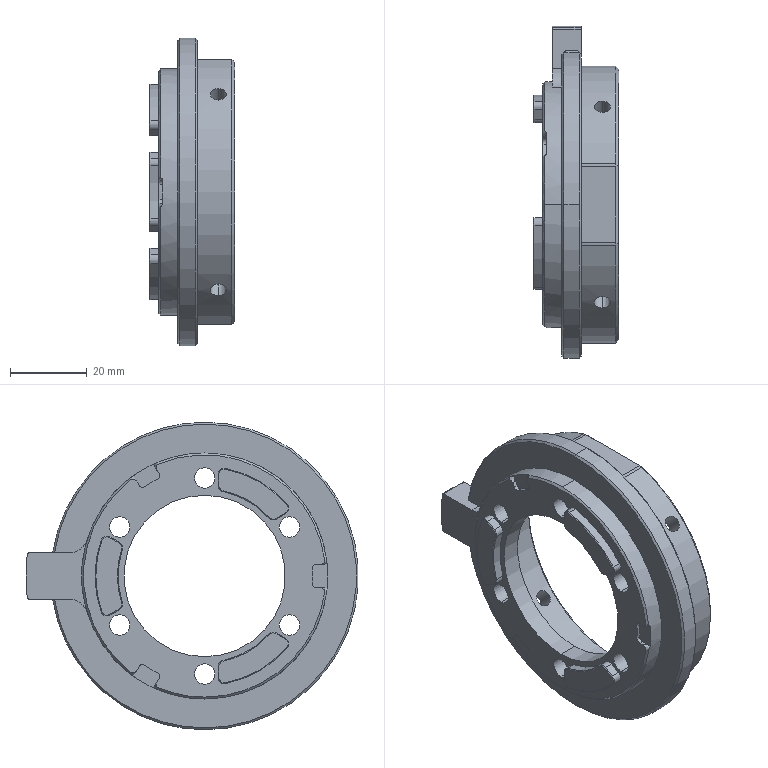NC program | NX | posted with a generic post | part box 22.3 x 86.5 x 80 mm
Lines 3855 to 5076 of 5076:
(ZLEVEL_PROFILE_COPY_1_COPY_COPY_1 , TOOL : D10JING)
N7696 T14 M6
N7698 G54
N7700 G17 G0 G90 X-1.456 Y13.884 S9500 M3
N7702 G43 Z30. H14
N7704 Z-21.3
N7706 G94 G1 Z-22.3 F1000.
N7708 X-2.389 Y15.5
N7710 G3 X-3.255 Y16. R1.
N7712 X-19.255 Y0. R16. F1200.
N7714 X-3.255 Y16. R-16.
N7716 X-4.121 Y15.5 R1.
N7718 G1 X-5.054 Y13.884
N7720 Z-21.3
N7722 G0 Z53.
N7724 X44.033 Y-12.821
N7726 Z-21.3
N7728 G1 Z-22.3 F1000.
N7730 X43.27 Y-11.5
N7732 G3 X42.404 Y-11. R1.
N7734 G1 X40.38 F1200.
N7736 G2 X40.38 Y11. R-45.
N7738 G1 X42.404
N7740 G2 X47.862 Y6.18 R5.5
N7742 X47.862 Y-6.18 R50.
N7744 X42.404 Y-11. R5.5
N7746 G3 X41.538 Y-11.5 R1.
N7748 G1 X41.912 Y-13.
N7750 Z-21.3
N7752 G0 Z30.
(ZLEVEL_PROFILE_COPY_1_COPY_COPY_1_COPY , TOOL : D10JING)
N7754 X-1.485 Y23.935
N7756 Z-11.7
N7758 G1 Z-12.7 F1000.
N7760 X-2.389 Y25.5
N7762 G3 X-3.255 Y26. R1.
N7764 X-29.255 Y0. R26. F1200.
N7766 X-3.255 Y26. R-26.
N7768 X-4.121 Y25.5 R1.
N7770 G1 X-5.025 Y23.935
N7772 Z-11.7
N7774 G0 Z30.
(FLOOR_WALL_1 , TOOL : D10JING)
N7776 X-21.493 Y2.989
N7778 Z-11.8
N7780 G1 Z-14.8 F1250.
N7782 X-21.755 Y0.
N7784 G3 X-20.35 Y-7.071 R18.5
N7786 G2 X-19.676 Y-9.481 R10.5
N7788 X-17.926 Y-11.269 R10.5
N7790 G3 X-5.679 Y-18.341 R18.5
N7792 G2 X-3.255 Y-18.962 R10.5
N7794 X-0.831 Y-18.341 R10.5
N7796 G3 X11.417 Y-11.269 R18.5
N7798 G2 X13.166 Y-9.481 R10.5
N7800 X13.84 Y-7.071 R10.5
N7802 G3 X13.84 Y7.071 R18.5
N7804 G2 X13.166 Y9.481 R10.5
N7806 X11.417 Y11.269 R10.5
N7808 G3 X-0.831 Y18.341 R18.5
N7810 G2 X-3.255 Y18.962 R10.5
N7812 X-5.679 Y18.341 R10.5
N7814 G3 X-17.926 Y11.269 R18.5
N7816 G2 X-19.676 Y9.481 R10.5
N7818 X-20.35 Y7.071 R10.5
N7820 G3 X-21.755 Y0. R18.5
N7822 G1 X-26.755
N7824 G3 X-24.971 Y-8.982 R23.5
N7826 G2 X-24.709 Y-12.387 R5.5
N7828 X-21.891 Y-14.315 R5.5
N7830 G3 X-6.334 Y-23.297 R23.5
N7832 G2 X-3.255 Y-24.774 R5.5
N7834 X-0.176 Y-23.297 R5.5
N7836 G3 X15.382 Y-14.315 R23.5
N7838 G2 X18.2 Y-12.387 R5.5
N7840 X18.461 Y-8.982 R5.5
N7842 G3 X18.461 Y8.982 R23.5
N7844 G2 X18.2 Y12.387 R5.5
N7846 X15.382 Y14.315 R5.5
N7848 G3 X-0.176 Y23.297 R23.5
N7850 G2 X-3.255 Y24.774 R5.5
N7852 X-6.334 Y23.297 R5.5
N7854 G3 X-21.891 Y14.315 R23.5
N7856 G2 X-24.709 Y12.387 R5.5
N7858 X-24.971 Y8.982 R5.5
N7860 G3 X-26.755 Y0. R23.5
N7862 G1 X-23.755
N7864 X-27.255
N7866 G3 X-25.433 Y-9.173 R24.
N7868 G2 X-25.338 Y-12.75 R5.
N7870 X-22.288 Y-14.62 R5.
N7872 G3 X-6.399 Y-23.793 R24.
N7874 G2 X-3.255 Y-25.5 R5.
N7876 X-0.11 Y-23.793 R5.
N7878 G3 X15.778 Y-14.62 R24.
N7880 G2 X18.829 Y-12.75 R5.
N7882 X18.923 Y-9.173 R5.
N7884 G3 X18.923 Y9.173 R24.
N7886 G2 X18.829 Y12.75 R5.
N7888 X15.778 Y14.62 R5.
N7890 G3 X-0.11 Y23.793 R24.
N7892 G2 X-3.255 Y25.5 R5.
N7894 X-6.399 Y23.793 R5.
N7896 G3 X-22.288 Y14.62 R24.
N7898 G2 X-25.338 Y12.75 R5.
N7900 X-25.433 Y9.173 R5.
N7902 G3 X-27.255 Y0. R24.
N7904 G1 X-24.255
N7906 Z-11.8
N7908 G0 Z30.
(FLOOR_WALL_1_COPY , TOOL : D10JING)
N7910 X42.135 Y14.
N7912 Z-6.8
N7914 G1 Z-9.8
N7916 X41.134 Y6.
N7918 X39.864
N7920 G2 X37.846 Y6.425 R5.
N7922 X37.846 Y-6.425 R41.6
N7924 X39.864 Y-6. R5.
N7926 G1 X42.404
N7928 G3 X42.9 Y-5.562 R0.5
N7930 X42.9 Y5.562 R45.
N7932 X42.404 Y6. R0.5
N7934 G1 X41.134
N7936 Y11.
N7938 X39.864
N7940 G3 X39.864 Y-11. R-44.5
N7942 G1 X42.404
N7944 G3 X47.862 Y-6.18 R5.5
N7946 X47.862 Y6.18 R50.
N7948 X42.404 Y11. R5.5
N7950 G1 X41.134
N7952 X39.55 Y10.608
N7954 X36.639 Y9.886
N7956 G2 X8.996 Y-39.232 R41.1
N7958 X6.581 Y-39.6 R8.1
N7960 G1 X-13.091
N7962 G2 X-15.505 Y-39.232 R8.1
N7964 X-15.505 Y39.232 R41.1
N7966 X-13.091 Y39.6 R8.1
N7968 G1 X6.581
N7970 G2 X8.996 Y39.232 R8.1
N7972 X36.639 Y9.886 R41.1
N7974 G1 X40.036 Y10.728
N7976 Z-6.8
N7978 G0 Z30.
N7980 M5
(ZLEVEL_PROFILE_1 , TOOL : D4R0.5)
N7982 T17 M6
N7984 G54
N7986 G17 G0 G90 X-2.557 Y28.19 S9500 M3
N7988 G43 Z30. H17
N7990 Z-11.4
N7992 G94 G1 Z-12.9 F2500.
N7994 X-2.908 Y28.799
N7996 G3 X-3.255 Y28.999 R0.4
N7998 X-32.253 Y0. R28.999
N8000 X-3.255 Y28.999 R-28.999
N8002 G1 Z-13.
N8004 G2 X25.744 Y0. R28.998
N8006 X-3.255 Y28.999 R-28.998
N8008 G1 Z-13.1
N8010 G3 X-32.253 Y0. R28.998
N8012 X-3.255 Y28.999 R-28.998
N8014 G1 Z-13.2
N8016 G2 X25.744 Y0. R28.998
N8018 X-3.255 Y28.999 R-28.998
N8020 G1 Z-13.3
N8022 G3 X-32.253 Y0. R28.998
N8024 X-3.255 Y28.999 R-28.998
N8026 G1 Y28.997 Z-13.4
N8028 G2 X-2.41 Y28.984 R28.997
N8030 G1 X-2.128 Y28.975
N8032 G2 X-1.001 Y28.909 R28.997
N8034 G1 X-0.72 Y28.886
N8036 G2 X0.655 Y28.732 R28.997
N8038 G1 X0.689 Y28.727
N8040 G2 X1.816 Y28.55 R28.997
N8042 G1 X2.097 Y28.498
N8044 G2 X3.224 Y28.264 R28.997
N8046 G1 X3.787 Y28.129
N8048 G2 X4.691 Y27.887 R28.997
N8050 G1 X5.196 Y27.738
N8052 G2 X5.759 Y27.56 R28.997
N8054 G1 X6.604 Y27.269
N8056 G2 X9.421 Y26.079 R28.997
N8058 G1 X9.985 Y25.797
N8060 G2 X10.829 Y25.346 R28.997
N8062 G1 X11.393 Y25.025
N8064 G2 X12.245 Y24.507 R28.997
N8066 G1 X12.52 Y24.33
N8068 G2 X13.506 Y23.662 R28.997
N8070 G1 X13.647 Y23.562
N8072 G2 X20.307 Y16.901 R28.997
N8074 G1 X20.407 Y16.761
N8076 G2 X21.076 Y15.775 R28.997
N8078 G1 X21.252 Y15.499
N8080 G2 X21.77 Y14.648 R28.997
N8082 G1 X22.092 Y14.084
N8084 G2 X22.543 Y13.24 R28.997
N8086 G1 X22.661 Y13.007
N8088 G2 X24.014 Y9.859 R28.997
N8090 G1 X24.069 Y9.703
N8092 X24.305 Y9.014
N8094 G2 X24.483 Y8.451 R28.997
N8096 G1 X24.632 Y7.946
N8098 G2 X24.874 Y7.042 R28.997
N8100 G1 X25.009 Y6.479
N8102 G2 X25.244 Y5.352 R28.997
N8104 G1 X25.295 Y5.07
N8106 G2 X25.472 Y3.944 R28.997
N8108 G1 X25.477 Y3.91
N8110 G2 X25.631 Y2.535 R28.997
N8112 G1 X25.654 Y2.253
N8114 G2 X25.72 Y1.127 R28.997
N8116 G1 X25.73 Y0.845
N8118 G2 X25.73 Y-0.845 R28.997
N8120 G1 X25.72 Y-1.127
N8122 G2 X25.654 Y-2.253 R28.997
N8124 G1 X25.631 Y-2.535
N8126 G2 X25.477 Y-3.91 R28.997
N8128 G1 X25.472 Y-3.944
N8130 G2 X25.295 Y-5.07 R28.997
N8132 G1 X25.244 Y-5.352
N8134 G2 X25.009 Y-6.479 R28.997
N8136 G1 X24.874 Y-7.042
N8138 G2 X24.632 Y-7.946 R28.997
N8140 G1 X24.483 Y-8.451
N8142 G2 X24.305 Y-9.014 R28.997
N8144 G1 X24.014 Y-9.859
N8146 G2 X22.661 Y-13.007 R28.997
N8148 G1 X22.543 Y-13.24
N8150 G2 X22.092 Y-14.084 R28.997
N8152 G1 X21.77 Y-14.648
N8154 G2 X21.252 Y-15.499 R28.997
N8156 G1 X21.076 Y-15.775
N8158 G2 X20.407 Y-16.761 R28.997
N8160 G1 X20.307 Y-16.901
N8162 G2 X13.647 Y-23.562 R28.997
N8164 G1 X13.506 Y-23.662
N8166 G2 X12.52 Y-24.33 R28.997
N8168 G1 X12.245 Y-24.507
N8170 G2 X11.393 Y-25.025 R28.997
N8172 G1 X10.829 Y-25.346
N8174 G2 X9.985 Y-25.797 R28.997
N8176 G1 X9.753 Y-25.915
N8178 G2 X6.604 Y-27.269 R28.997
N8180 G1 X6.449 Y-27.323
N8182 X5.759 Y-27.56
N8184 G2 X5.196 Y-27.738 R28.997
N8186 G1 X4.691 Y-27.887
N8188 G2 X3.787 Y-28.129 R28.997
N8190 G1 X3.224 Y-28.264
N8192 G2 X2.097 Y-28.498 R28.997
N8194 G1 X1.816 Y-28.55
N8196 G2 X0.689 Y-28.727 R28.997
N8198 G1 X0.655 Y-28.732
N8200 G2 X-0.72 Y-28.886 R28.997
N8202 G1 X-1.001 Y-28.909
N8204 G2 X-2.128 Y-28.975 R28.997
N8206 G1 X-2.41 Y-28.984
N8208 G2 X-4.1 Y-28.984 R28.997
N8210 G1 X-4.382 Y-28.975
N8212 G2 X-5.508 Y-28.909 R28.997
N8214 G1 X-5.79 Y-28.886
N8216 G2 X-7.164 Y-28.732 R28.997
N8218 G1 X-7.198 Y-28.727
N8220 G2 X-8.325 Y-28.55 R28.997
N8222 G1 X-8.607 Y-28.498
N8224 G2 X-9.734 Y-28.264 R28.997
N8226 G1 X-10.297 Y-28.129
N8228 G2 X-11.2 Y-27.887 R28.997
N8230 G1 X-11.705 Y-27.738
N8232 G2 X-12.269 Y-27.56 R28.997
N8234 G1 X-13.114 Y-27.269
N8236 G2 X-16.262 Y-25.915 R28.997
N8238 G1 X-16.495 Y-25.797
N8240 G2 X-17.339 Y-25.346 R28.997
N8242 G1 X-17.903 Y-25.025
N8244 G2 X-18.754 Y-24.507 R28.997
N8246 G1 X-19.03 Y-24.33
N8248 G2 X-20.016 Y-23.662 R28.997
N8250 G1 X-20.156 Y-23.562
N8252 G2 X-26.816 Y-16.901 R28.997
N8254 G1 X-26.916 Y-16.761
N8256 G2 X-27.585 Y-15.775 R28.997
N8258 G1 X-27.761 Y-15.499
N8260 G2 X-28.28 Y-14.648 R28.997
N8262 G1 X-28.601 Y-14.084
N8264 G2 X-29.052 Y-13.24 R28.997
N8266 G1 X-29.334 Y-12.676
N8268 G2 X-30.524 Y-9.859 R28.997
N8270 G1 X-30.578 Y-9.703
N8272 X-30.815 Y-9.014
N8274 G2 X-30.993 Y-8.451 R28.997
N8276 G1 X-31.142 Y-7.946
N8278 G2 X-31.383 Y-7.042 R28.997
N8280 G1 X-31.518 Y-6.479
N8282 G2 X-31.753 Y-5.352 R28.997
N8284 G1 X-31.805 Y-5.07
N8286 G2 X-31.982 Y-3.944 R28.997
N8288 G1 X-31.987 Y-3.91
N8290 G2 X-32.14 Y-2.535 R28.997
N8292 G1 X-32.164 Y-2.253
N8294 G2 X-32.23 Y-1.127 R28.997
N8296 G1 X-32.239 Y-0.845
N8298 G2 X-32.239 Y0.845 R28.997
N8300 G1 X-32.23 Y1.127
N8302 G2 X-31.987 Y3.91 R28.997
N8304 G1 X-31.982 Y3.944
N8306 G2 X-31.805 Y5.07 R28.997
N8308 G1 X-31.753 Y5.352
N8310 G2 X-31.518 Y6.479 R28.997
N8312 G1 X-31.383 Y7.042
N8314 G2 X-31.142 Y7.946 R28.997
N8316 G1 X-30.993 Y8.451
N8318 G2 X-30.815 Y9.014 R28.997
N8320 G1 X-30.524 Y9.859
N8322 G2 X-29.334 Y12.676 R28.997
N8324 G1 X-29.052 Y13.24
N8326 G2 X-28.601 Y14.084 R28.997
N8328 G1 X-28.28 Y14.648
N8330 G2 X-27.761 Y15.499 R28.997
N8332 G1 X-27.585 Y15.775
N8334 G2 X-26.916 Y16.761 R28.997
N8336 G1 X-26.816 Y16.901
N8338 G2 X-20.156 Y23.562 R28.997
N8340 G1 X-20.016 Y23.662
N8342 G2 X-19.03 Y24.33 R28.997
N8344 G1 X-18.754 Y24.507
N8346 G2 X-17.903 Y25.025 R28.997
N8348 G1 X-17.339 Y25.346
N8350 G2 X-16.495 Y25.797 R28.997
N8352 G1 X-15.931 Y26.079
N8354 G2 X-13.114 Y27.269 R28.997
N8356 G1 X-12.958 Y27.323
N8358 X-12.269 Y27.56
N8360 G2 X-11.705 Y27.738 R28.997
N8362 G1 X-11.2 Y27.887
N8364 G2 X-10.297 Y28.129 R28.997
N8366 G1 X-9.734 Y28.264
N8368 G2 X-8.607 Y28.498 R28.997
N8370 G1 X-8.325 Y28.55
N8372 G2 X-7.198 Y28.727 R28.997
N8374 G1 X-7.164 Y28.732
N8376 G2 X-5.79 Y28.886 R28.997
N8378 G1 X-5.508 Y28.909
N8380 G2 X-4.382 Y28.975 R28.997
N8382 G1 X-4.1 Y28.984
N8384 G2 X-3.255 Y28.997 R28.997
N8386 G1 Y28.987 Z-13.499
N8388 G3 X-32.242 Y0. R28.987
N8390 X-3.255 Y28.987 R-28.987
N8392 G1 Y28.979 Z-13.549
N8394 Y28.97 Z-13.598
N8396 X-3.246
N8398 G2 X25.715 Y-0.009 R28.97
N8400 X-3.255 Y28.97 R-28.97
N8402 G1 Y28.959 Z-13.646
N8404 Y28.947 Z-13.695
N8406 X-3.264
N8408 G3 X-32.202 Y-0.009 R28.947
N8410 X-3.255 Y28.947 R-28.947
N8412 G1 Y28.933 Z-13.743
N8414 Y28.918 Z-13.79
N8416 G2 X25.663 Y0. R28.918
N8418 X-3.255 Y28.918 R-28.918
N8420 G1 Y28.901 Z-13.837
N8422 Y28.882 Z-13.884
N8424 X-3.264
N8426 G3 X-32.137 Y-0.009 R28.882
N8428 X-3.255 Y28.882 R-28.882
N8430 G1 Y28.862 Z-13.929
N8432 Y28.84 Z-13.974
N8434 G2 X25.585 Y0. R28.84
N8436 X-3.255 Y28.84 R-28.84
N8438 G1 Y28.817 Z-14.018
N8440 Y28.792 Z-14.062
N8442 X-3.264
N8444 G3 X-32.047 Y-0.009 R28.792
N8446 X-3.255 Y28.792 R-28.792
N8448 G1 Y28.766 Z-14.104
N8450 Y28.739 Z-14.146
N8452 G2 X25.484 Y0. R28.739
N8454 X-3.255 Y28.739 R-28.739
N8456 G1 Y28.71 Z-14.186
N8458 Y28.68 Z-14.226
N8460 G3 X-31.935 Y0. R28.68
N8462 X-3.255 Y28.68 R-28.68
N8464 G1 Y28.649 Z-14.265
N8466 Y28.613 Z-14.303
N8468 X-2.904
N8470 G2 X-2.904 Y-28.613 R28.616
N8472 G1 X-3.605
N8474 G2 X-3.605 Y28.613 R28.616
N8476 G1 X-3.255
N8478 Y28.579 Z-14.339
N8480 Y28.547 Z-14.374
N8482 G3 X-31.801 Y0. R28.547
N8484 X-3.255 Y28.547 R-28.547
N8486 G1 Y28.512 Z-14.408
N8488 Y28.473 Z-14.441
N8490 G2 X25.218 Y0. R28.473
N8492 X-3.255 Y28.473 R-28.473
N8494 G1 Y28.448 Z-14.472
N8496 X-3.254 Y28.404 Z-14.503
N8498 G3 X-4.105 Y28.382 R21.334
N8500 G1 X-5.013 Y28.341
N8502 G3 X-26.917 Y15.697 R28.396
N8504 G1 X-27.042 Y15.493
N8506 X-27.198 Y15.263
N8508 G3 X-28.662 Y12.676 R21.533
N8510 G1 X-28.678 Y12.647
N8512 G3 X-28.678 Y-12.647 R28.396
N8514 G1 X-28.662 Y-12.676
N8516 G3 X-27.04 Y-15.493 R20.666
N8518 G1 X-26.917 Y-15.697
N8520 G3 X-5.014 Y-28.341 R28.396
N8522 X-2.449 Y-28.384 R20.768
N8524 G1 X-1.496 Y-28.341
N8526 G3 X20.407 Y-15.697 R28.396
N8528 G1 X20.532 Y-15.493
N8530 G3 X21.639 Y-13.67 R15.292
N8532 G1 X22.152 Y-12.676
N8534 X22.169 Y-12.647
N8536 G3 X22.169 Y12.647 R28.396
N8538 G1 X22.153 Y12.676
N8540 G3 X20.53 Y15.493 R20.668
N8542 G1 X20.408 Y15.697
N8544 G3 X-1.496 Y28.341 R28.396
N8546 X-3.254 Y28.404 R21.334
N8548 G1 X-3.255 Y28.386 Z-14.532
N8550 Y28.348 Z-14.56
N8552 X-1.221 Y28.241
N8554 G2 X20.186 Y15.882 R28.314
N8556 G1 X21.181 Y14.366
N8558 X21.349 Y14.084
N8560 X22.097 Y12.598
N8562 X22.219 Y12.359
N8564 G2 X22.22 Y-12.357 R28.314
N8566 G1 X21.35 Y-14.084
N8568 X21.179 Y-14.366
N8570 X20.186 Y-15.882
N8572 G2 X-1.221 Y-28.241 R28.314
N8574 G1 X-3.255 Y-28.35
N8576 X-5.289 Y-28.241
N8578 G2 X-26.695 Y-15.882 R28.314
N8580 G1 X-27.69 Y-14.366
N8582 X-27.859 Y-14.084
N8584 X-28.005 Y-13.803
N8586 X-28.606 Y-12.598
N8588 X-28.729 Y-12.359
N8590 G2 X-28.73 Y12.357 R28.314
N8592 G1 X-27.86 Y14.084
N8594 X-27.689 Y14.366
N8596 X-26.695 Y15.882
N8598 G2 X-5.288 Y28.241 R28.314
N8600 G1 X-3.255 Y28.348
N8602 Y28.321 Z-14.584
N8604 Y28.288 Z-14.607
N8606 X-5.508 Y28.141
N8608 X-5.521 Y28.144
N8610 G3 X-26.497 Y16.033 R28.235
N8612 G2 X-27.791 Y14.084 R361.16
N8614 X-28.76 Y12.112 R86.463
N8616 G3 X-28.761 Y-12.112 R28.235
N8618 G1 X-28.623 Y-12.394
N8620 G2 X-28.246 Y-13.156 R8.904
N8622 G3 X-27.104 Y-15.111 R9.73
N8624 G1 X-27.029 Y-15.211
N8626 X-26.497 Y-16.033
N8628 G3 X-5.519 Y-28.144 R28.235
N8630 G1 X-3.255 Y-28.29
N8632 G2 X-1.895 Y-28.203 R42.489
N8634 G3 X19.987 Y-16.033 R28.235
N8636 G2 X21.281 Y-14.084 R362.689
N8638 X22.251 Y-12.112 R86.463
N8640 G3 X22.251 Y12.112 R28.235
N8642 G1 X22.113 Y12.394
N8644 G2 X21.736 Y13.155 R8.904
N8646 G3 X20.594 Y15.112 R9.733
N8648 G1 X20.519 Y15.211
N8650 X19.987 Y16.033
N8652 G3 X-0.991 Y28.144 R28.235
N8654 G1 X-2.973 Y28.273
N8656 X-3.255 Y28.288
N8658 Y28.264 Z-14.625
N8660 Y28.232 Z-14.643
N8662 X-0.775 Y28.059
N8664 G2 X19.817 Y16.159 R28.168
N8666 G1 X19.823 Y16.142
N8668 X21.217 Y14.084
N8670 X22.267 Y11.919
N8672 G2 X22.267 Y-11.92 R28.168
N8674 G1 X22.167 Y-12.112
N8676 X21.356 Y-13.803
N8678 X21.219 Y-14.084
N8680 X19.843 Y-16.115
N8682 X19.829 Y-16.142
N8684 G2 X-0.774 Y-28.059 R28.168
N8686 G1 X-3.255 Y-28.232
N8688 X-5.735 Y-28.059
N8690 G2 X-26.328 Y-16.158 R28.168
N8692 G1 X-26.334 Y-16.141
N8694 X-27.726 Y-14.084
N8696 X-28.777 Y-11.919
N8698 G2 X-28.776 Y11.92 R28.168
N8700 G1 X-28.677 Y12.112
N8702 X-27.866 Y13.803
N8704 X-27.729 Y14.084
N8706 X-26.353 Y16.115
N8708 X-26.338 Y16.144
N8710 G2 X-5.735 Y28.059 R28.168
N8712 G1 X-3.255 Y28.232
N8714 Y28.207 Z-14.661
N8716 Y28.176 Z-14.679
N8718 X-5.508 Y27.973
N8720 X-5.889 Y27.967
N8722 G3 X-26.158 Y16.265 R28.091
N8724 G1 X-27.655 Y14.084
N8726 X-28.802 Y11.682
N8728 G3 X-28.802 Y-11.682 R28.091
N8730 G1 X-27.656 Y-14.084
N8732 X-26.283 Y-16.056
N8734 X-26.158 Y-16.265
N8736 G3 X-5.889 Y-27.967 R28.091
N8738 G1 X-5.877 Y-27.962
N8740 X-3.255 Y-28.174
N8742 X-1.001 Y-27.972
N8744 X-0.621 Y-27.967
N8746 G3 X19.649 Y-16.265 R28.091
N8748 G1 X21.146 Y-14.084
N8750 X22.292 Y-11.682
N8752 G3 X22.292 Y11.682 R28.091
N8754 G1 X21.146 Y14.084
N8756 X19.773 Y16.056
N8758 X19.648 Y16.265
N8760 G3 X-0.621 Y27.967 R28.091
N8762 G1 X-0.72 Y27.966
N8764 X-3.255 Y28.176
N8766 Y28.133 Z-14.696
N8768 Y28.088 Z-14.714
N8770 X-0.438 Y27.859
N8772 G2 X19.449 Y16.389 R28.001
N8774 G1 X19.562 Y16.209
N8776 X20.97 Y14.193
N8778 X21.052 Y14.084
N8780 X22.273 Y11.489
N8782 X22.287 Y11.475
N8784 G2 X22.287 Y-11.475 R28.001
N8786 G1 X21.19 Y-13.803
N8788 X20.97 Y-14.231
N8790 X20.865 Y-14.366
N8792 X19.459 Y-16.363
N8794 X19.449 Y-16.389
N8796 G2 X-0.438 Y-27.859 R28.001
N8798 G1 X-3.255 Y-28.092
N8800 X-6.072 Y-27.859
N8802 G2 X-25.958 Y-16.389 R28.001
N8804 G1 X-26.071 Y-16.209
N8806 X-27.48 Y-14.195
N8808 X-27.563 Y-14.084
N8810 X-28.783 Y-11.489
N8812 X-28.796 Y-11.475
N8814 G2 X-28.796 Y11.475 R28.001
N8816 G1 X-27.7 Y13.803
N8818 X-27.48 Y14.231
N8820 X-27.374 Y14.366
N8822 X-25.969 Y16.363
N8824 X-25.958 Y16.389
N8826 G2 X-6.072 Y27.859 R28.001
N8828 G1 X-3.255 Y28.088
N8830 Y28.035 Z-14.732
N8832 Y27.919 Z-14.75
N8834 G3 X-6.291 Y27.709 R22.026
N8836 G1 X-6.314 Y27.716
N8838 G3 X-25.737 Y16.495 R27.884
N8840 G1 X-27.566 Y13.803
N8842 X-27.713 Y13.521
N8844 X-28.786 Y11.21
N8846 G3 X-28.786 Y-11.21 R27.884
N8848 G1 X-27.592 Y-13.803
N8850 X-27.48 Y-13.993
N8852 X-25.737 Y-16.495
N8854 G3 X-6.314 Y-27.716 R27.884
N8856 G1 X-6.291 Y-27.709
N8858 X-3.255 Y-27.988
N8860 X-0.196 Y-27.716
N8862 G3 X19.227 Y-16.495 R27.884
N8864 G1 X21.056 Y-13.803
N8866 X21.203 Y-13.521
N8868 X22.276 Y-11.21
N8870 G3 X22.276 Y11.21 R27.884
N8872 G1 X21.073 Y13.803
N8874 X20.97 Y13.98
N8876 X19.227 Y16.495
N8878 G3 X-0.196 Y27.716 R27.884
N8880 G1 X-0.218 Y27.709
N8882 G3 X-3.255 Y27.919 R22.026
N8884 X-3.601 Y27.719 R0.4
N8886 G1 X-3.954 Y27.108
N8888 Z-13.25
N8890 G0 Z30.
N8892 M5
(ZLEVEL_PROFILE_COPY , TOOL : D2)
N8894 T18 M6
N8896 G54
N8898 G17 G0 G90 X40.167 Y-7.4 S9500 M3
N8900 G43 Z30. H18
N8902 Z-9.947
N8904 G94 G1 X39.994 Y-7.1 F1000.
N8906 G3 X39.821 Y-7. R0.2
N8908 G1 X36.785
N8910 G2 X36.179 Y-9.856 R40.647
N8912 G3 X36.234 Y-10.048 R0.2
N8914 G1 X36.482 Y-10.288
N8916 G0 X40.319 Y-7.4 Z-10.094
N8918 G1 X40.145 Y-7.1
N8920 G3 X39.972 Y-7. R0.2
N8922 G1 X36.934
N8924 G2 X36.33 Y-9.859 R40.794
N8926 G3 X36.385 Y-10.051 R0.2
N8928 G1 X36.633 Y-10.291
N8930 G0 X40.47 Y-7.4 Z-10.241
N8932 G1 X40.297 Y-7.1
N8934 G3 X40.124 Y-7. R0.2
N8936 G1 X37.083
N8938 G2 X36.481 Y-9.862 R40.941
N8940 G3 X36.536 Y-10.054 R0.2
N8942 G1 X36.784 Y-10.294
N8944 G0 X40.529 Y-7.4 Z-10.388
N8946 G1 X40.356 Y-7.1
N8948 G3 X40.183 Y-7. R0.2
N8950 G1 X37.141
N8952 X37.122 Y-7.122
N8954 G2 X36.544 Y-9.853 R41.
N8956 G3 X36.599 Y-10.046 R0.2
N8958 G1 X36.847 Y-10.285
N8960 G0 X40.53 Y-7.4 Z-10.535
N8962 G1 X40.357 Y-7.1
N8964 G3 X40.184 Y-7. R0.2
N8966 G1 X37.142
N8968 X37.122 Y-7.122
N8970 G2 X36.542 Y-9.859 R41.
N8972 G3 X36.598 Y-10.051 R0.2
N8974 G1 X36.846 Y-10.291
N8976 G0 X40.531 Y-7.4 Z-10.682
N8978 G1 X40.357 Y-7.1
N8980 G3 X40.184 Y-7. R0.2
N8982 G1 X37.143
N8984 G2 X36.542 Y-9.861 R41.
N8986 G3 X36.597 Y-10.054 R0.2
N8988 G1 X36.845 Y-10.293
N8990 G0 X40.531 Y-7.4 Z-10.829
N8992 G1 X40.357 Y-7.1
N8994 G3 X40.184 Y-7. R0.2
N8996 G1 X37.143
N8998 G2 X36.542 Y-9.861 R41.
N9000 G3 X36.597 Y-10.054 R0.2
N9002 G1 X36.845 Y-10.293
N9004 G0 X40.531 Y-7.4 Z-10.976
N9006 G1 X40.357 Y-7.1
N9008 G3 X40.184 Y-7. R0.2
N9010 G1 X37.143
N9012 G2 X36.542 Y-9.861 R41.
N9014 G3 X36.597 Y-10.054 R0.2
N9016 G1 X36.845 Y-10.293
N9018 G0 X40.531 Y-7.4 Z-11.124
N9020 G1 X40.357 Y-7.1
N9022 G3 X40.184 Y-7. R0.2
N9024 G1 X37.143
N9026 G2 X36.542 Y-9.861 R41.
N9028 G3 X36.597 Y-10.054 R0.2
N9030 G1 X36.845 Y-10.293
N9032 G0 X40.531 Y-7.4 Z-11.271
N9034 G1 X40.357 Y-7.1
N9036 G3 X40.184 Y-7. R0.2
N9038 G1 X37.143
N9040 G2 X36.542 Y-9.861 R41.
N9042 G3 X36.597 Y-10.054 R0.2
N9044 G1 X36.845 Y-10.293
N9046 G0 X40.531 Y-7.4 Z-11.418
N9048 G1 X40.357 Y-7.1
N9050 G3 X40.184 Y-7. R0.2
N9052 G1 X37.143
N9054 G2 X36.542 Y-9.861 R41.
N9056 G3 X36.597 Y-10.054 R0.2
N9058 G1 X36.845 Y-10.293
N9060 G0 X40.531 Y-7.4 Z-11.565
N9062 G1 X40.357 Y-7.1
N9064 G3 X40.184 Y-7. R0.2
N9066 G1 X37.143
N9068 G2 X36.542 Y-9.861 R41.
N9070 G3 X36.597 Y-10.054 R0.2
N9072 G1 X36.845 Y-10.293
N9074 G0 X40.531 Y-7.4 Z-11.712
N9076 G1 X40.357 Y-7.1
N9078 G3 X40.184 Y-7. R0.2
N9080 G1 X37.143
N9082 G2 X36.542 Y-9.861 R41.
N9084 G3 X36.597 Y-10.054 R0.2
N9086 G1 X36.845 Y-10.293
N9088 G0 X40.531 Y-7.4 Z-11.859
N9090 G1 X40.357 Y-7.1
N9092 G3 X40.184 Y-7. R0.2
N9094 G1 X37.143
N9096 G2 X36.542 Y-9.861 R41.
N9098 G3 X36.597 Y-10.054 R0.2
N9100 G1 X36.845 Y-10.293
N9102 G0 X40.531 Y-7.4 Z-12.006
N9104 G1 X40.357 Y-7.1
N9106 G3 X40.184 Y-7. R0.2
N9108 G1 X37.143
N9110 G2 X36.542 Y-9.861 R41.
N9112 G3 X36.597 Y-10.054 R0.2
N9114 G1 X36.845 Y-10.293
N9116 G0 X40.531 Y-7.4 Z-12.153
N9118 G1 X40.357 Y-7.1
N9120 G3 X40.184 Y-7. R0.2
N9122 G1 X37.143
N9124 G2 X36.542 Y-9.861 R41.
N9126 G3 X36.597 Y-10.054 R0.2
N9128 G1 X36.845 Y-10.293
N9130 G0 X40.531 Y-7.4 Z-12.3
N9132 G1 X40.357 Y-7.1
N9134 G3 X40.184 Y-7. R0.2
N9136 G1 X37.143
N9138 G2 X36.542 Y-9.861 R41.
N9140 G3 X36.597 Y-10.054 R0.2
N9142 G1 X36.845 Y-10.293
N9144 G0 X40.531 Y-7.4 Z-12.447
N9146 G1 X40.357 Y-7.1
N9148 G3 X40.184 Y-7. R0.2
N9150 G1 X37.143
N9152 G2 X36.542 Y-9.861 R41.
N9154 G3 X36.597 Y-10.054 R0.2
N9156 G1 X36.845 Y-10.293
N9158 G0 X40.531 Y-7.4 Z-12.594
N9160 G1 X40.357 Y-7.1
N9162 G3 X40.184 Y-7. R0.2
N9164 G1 X37.143
N9166 G2 X36.542 Y-9.861 R41.
N9168 G3 X36.597 Y-10.054 R0.2
N9170 G1 X36.845 Y-10.293
N9172 G0 X40.531 Y-7.4 Z-12.741
N9174 G1 X40.357 Y-7.1
N9176 G3 X40.184 Y-7. R0.2
N9178 G1 X37.143
N9180 G2 X36.542 Y-9.861 R41.
N9182 G3 X36.597 Y-10.054 R0.2
N9184 G1 X36.845 Y-10.293
N9186 G0 X40.531 Y-7.4 Z-12.888
N9188 G1 X40.357 Y-7.1
N9190 G3 X40.184 Y-7. R0.2
N9192 G1 X37.143
N9194 G2 X36.542 Y-9.861 R41.
N9196 G3 X36.597 Y-10.054 R0.2
N9198 G1 X36.845 Y-10.293
N9200 G0 X40.531 Y-7.4 Z-13.035
N9202 G1 X40.357 Y-7.1
N9204 G3 X40.184 Y-7. R0.2
N9206 G1 X37.143
N9208 G2 X36.542 Y-9.861 R41.
N9210 G3 X36.597 Y-10.054 R0.2
N9212 G1 X36.845 Y-10.293
N9214 G0 X40.531 Y-7.4 Z-13.182
N9216 G1 X40.357 Y-7.1
N9218 G3 X40.184 Y-7. R0.2
N9220 G1 X37.143
N9222 G2 X36.542 Y-9.861 R41.
N9224 G3 X36.597 Y-10.054 R0.2
N9226 G1 X36.845 Y-10.293
N9228 G0 X40.531 Y-7.4 Z-13.329
N9230 G1 X40.357 Y-7.1
N9232 G3 X40.184 Y-7. R0.2
N9234 G1 X37.143
N9236 G2 X36.542 Y-9.861 R41.
N9238 G3 X36.597 Y-10.054 R0.2
N9240 G1 X36.845 Y-10.293
N9242 G0 X40.531 Y-7.4 Z-13.476
N9244 G1 X40.357 Y-7.1
N9246 G3 X40.184 Y-7. R0.2
N9248 G1 X37.143
N9250 G2 X36.542 Y-9.861 R41.
N9252 G3 X36.597 Y-10.054 R0.2
N9254 G1 X36.845 Y-10.293
N9256 G0 X40.531 Y-7.4 Z-13.624
N9258 G1 X40.357 Y-7.1
N9260 G3 X40.184 Y-7. R0.2
N9262 G1 X37.143
N9264 G2 X36.542 Y-9.861 R41.
N9266 G3 X36.597 Y-10.054 R0.2
N9268 G1 X36.845 Y-10.293
N9270 G0 X40.531 Y-7.4 Z-13.771
N9272 G1 X40.357 Y-7.1
N9274 G3 X40.184 Y-7. R0.2
N9276 G1 X37.143
N9278 G2 X36.542 Y-9.861 R41.
N9280 G3 X36.597 Y-10.054 R0.2
N9282 G1 X36.845 Y-10.293
N9284 G0 X40.531 Y-7.4 Z-13.918
N9286 G1 X40.357 Y-7.1
N9288 G3 X40.184 Y-7. R0.2
N9290 G1 X37.143
N9292 G2 X36.542 Y-9.861 R41.
N9294 G3 X36.597 Y-10.054 R0.2
N9296 G1 X36.845 Y-10.293
N9298 G0 X40.531 Y-7.4 Z-14.065
N9300 G1 X40.357 Y-7.1
N9302 G3 X40.184 Y-7. R0.2
N9304 G1 X37.143
N9306 G2 X36.542 Y-9.861 R41.
N9308 G3 X36.597 Y-10.054 R0.2
N9310 G1 X36.845 Y-10.293
N9312 G0 X40.531 Y-7.4 Z-14.212
N9314 G1 X40.357 Y-7.1
N9316 G3 X40.184 Y-7. R0.2
N9318 G1 X37.143
N9320 G2 X36.542 Y-9.861 R41.
N9322 G3 X36.597 Y-10.054 R0.2
N9324 G1 X36.845 Y-10.293
N9326 G0 X40.531 Y-7.4 Z-14.359
N9328 G1 X40.357 Y-7.1
N9330 G3 X40.184 Y-7. R0.2
N9332 G1 X37.143
N9334 G2 X36.542 Y-9.861 R41.
N9336 G3 X36.597 Y-10.054 R0.2
N9338 G1 X36.845 Y-10.293
N9340 G0 X40.531 Y-7.4 Z-14.506
N9342 G1 X40.357 Y-7.1
N9344 G3 X40.184 Y-7. R0.2
N9346 G1 X37.143
N9348 G2 X36.542 Y-9.861 R41.
N9350 G3 X36.597 Y-10.054 R0.2
N9352 G1 X36.845 Y-10.293
N9354 G0 X40.531 Y-7.4 Z-14.653
N9356 G1 X40.357 Y-7.1
N9358 G3 X40.184 Y-7. R0.2
N9360 G1 X37.143
N9362 G2 X36.542 Y-9.861 R41.
N9364 G3 X36.597 Y-10.054 R0.2
N9366 G1 X36.845 Y-10.293
N9368 G0 X40.531 Y-7.4 Z-14.8
N9370 G1 X40.357 Y-7.1
N9372 G3 X40.184 Y-7. R0.2
N9374 G1 X37.143
N9376 G2 X36.542 Y-9.861 R41.
N9378 G3 X36.597 Y-10.054 R0.2
N9380 G1 X36.845 Y-10.293
N9382 G0 Z30.
N9384 X36.482 Y10.288
N9386 Z-9.947
N9388 G1 X36.234 Y10.048
N9390 G3 X36.179 Y9.856 R0.2
N9392 G2 X36.785 Y7. R40.647
N9394 G1 X39.821
N9396 G3 X39.994 Y7.1 R0.2
N9398 G1 X40.167 Y7.4
N9400 G0 X36.633 Y10.291 Z-10.094
N9402 G1 X36.385 Y10.051
N9404 G3 X36.33 Y9.859 R0.2
N9406 G2 X36.934 Y7. R40.794
N9408 G1 X39.972
N9410 G3 X40.145 Y7.1 R0.2
N9412 G1 X40.319 Y7.4
N9414 G0 X36.784 Y10.294 Z-10.241
N9416 G1 X36.536 Y10.054
N9418 G3 X36.481 Y9.862 R0.2
N9420 G2 X37.083 Y7. R40.941
N9422 G1 X40.124
N9424 G3 X40.297 Y7.1 R0.2
N9426 G1 X40.47 Y7.4
N9428 G0 X36.847 Y10.285 Z-10.388
N9430 G1 X36.599 Y10.046
N9432 G3 X36.544 Y9.853 R0.2
N9434 G2 X37.122 Y7.122 R41.
N9436 G1 X37.141 Y7.
N9438 X40.183
N9440 G3 X40.356 Y7.1 R0.2
N9442 G1 X40.529 Y7.4
N9444 G0 X36.846 Y10.291 Z-10.535
N9446 G1 X36.598 Y10.051
N9448 G3 X36.542 Y9.859 R0.2
N9450 G2 X37.122 Y7.122 R41.
N9452 G1 X37.142 Y7.
N9454 X40.184
N9456 G3 X40.357 Y7.1 R0.2
N9458 G1 X40.53 Y7.4
N9460 G0 X36.845 Y10.293 Z-10.682
N9462 G1 X36.597 Y10.054
N9464 G3 X36.542 Y9.861 R0.2
N9466 G2 X37.143 Y7. R41.
N9468 G1 X40.184
N9470 G3 X40.357 Y7.1 R0.2
N9472 G1 X40.531 Y7.4
N9474 G0 X36.845 Y10.293 Z-10.829
N9476 G1 X36.597 Y10.054
N9478 G3 X36.542 Y9.861 R0.2
N9480 G2 X37.143 Y7. R41.
N9482 G1 X40.184
N9484 G3 X40.357 Y7.1 R0.2
N9486 G1 X40.531 Y7.4
N9488 G0 X36.845 Y10.293 Z-10.976
N9490 G1 X36.597 Y10.054
N9492 G3 X36.542 Y9.861 R0.2
N9494 G2 X37.143 Y7. R41.
N9496 G1 X40.184
N9498 G3 X40.357 Y7.1 R0.2
N9500 G1 X40.531 Y7.4
N9502 G0 X36.845 Y10.293 Z-11.124
N9504 G1 X36.597 Y10.054
N9506 G3 X36.542 Y9.861 R0.2
N9508 G2 X37.143 Y7. R41.
N9510 G1 X40.184
N9512 G3 X40.357 Y7.1 R0.2
N9514 G1 X40.531 Y7.4
N9516 G0 X36.845 Y10.293 Z-11.271
N9518 G1 X36.597 Y10.054
N9520 G3 X36.542 Y9.861 R0.2
N9522 G2 X37.143 Y7. R41.
N9524 G1 X40.184
N9526 G3 X40.357 Y7.1 R0.2
N9528 G1 X40.531 Y7.4
N9530 G0 X36.845 Y10.293 Z-11.418
N9532 G1 X36.597 Y10.054
N9534 G3 X36.542 Y9.861 R0.2
N9536 G2 X37.143 Y7. R41.
N9538 G1 X40.184
N9540 G3 X40.357 Y7.1 R0.2
N9542 G1 X40.531 Y7.4
N9544 G0 X36.845 Y10.293 Z-11.565
N9546 G1 X36.597 Y10.054
N9548 G3 X36.542 Y9.861 R0.2
N9550 G2 X37.143 Y7. R41.
N9552 G1 X40.184
N9554 G3 X40.357 Y7.1 R0.2
N9556 G1 X40.531 Y7.4
N9558 G0 X36.845 Y10.293 Z-11.712
N9560 G1 X36.597 Y10.054
N9562 G3 X36.542 Y9.861 R0.2
N9564 G2 X37.143 Y7. R41.
N9566 G1 X40.184
N9568 G3 X40.357 Y7.1 R0.2
N9570 G1 X40.531 Y7.4
N9572 G0 X36.845 Y10.293 Z-11.859
N9574 G1 X36.597 Y10.054
N9576 G3 X36.542 Y9.861 R0.2
N9578 G2 X37.143 Y7. R41.
N9580 G1 X40.184
N9582 G3 X40.357 Y7.1 R0.2
N9584 G1 X40.531 Y7.4
N9586 G0 X36.845 Y10.293 Z-12.006
N9588 G1 X36.597 Y10.054
N9590 G3 X36.542 Y9.861 R0.2
N9592 G2 X37.143 Y7. R41.
N9594 G1 X40.184
N9596 G3 X40.357 Y7.1 R0.2
N9598 G1 X40.531 Y7.4
N9600 G0 X36.845 Y10.293 Z-12.153
N9602 G1 X36.597 Y10.054
N9604 G3 X36.542 Y9.861 R0.2
N9606 G2 X37.143 Y7. R41.
N9608 G1 X40.184
N9610 G3 X40.357 Y7.1 R0.2
N9612 G1 X40.531 Y7.4
N9614 G0 X36.845 Y10.293 Z-12.3
N9616 G1 X36.597 Y10.054
N9618 G3 X36.542 Y9.861 R0.2
N9620 G2 X37.143 Y7. R41.
N9622 G1 X40.184
N9624 G3 X40.357 Y7.1 R0.2
N9626 G1 X40.531 Y7.4
N9628 G0 X36.845 Y10.293 Z-12.447
N9630 G1 X36.597 Y10.054
N9632 G3 X36.542 Y9.861 R0.2
N9634 G2 X37.143 Y7. R41.
N9636 G1 X40.184
N9638 G3 X40.357 Y7.1 R0.2
N9640 G1 X40.531 Y7.4
N9642 G0 X36.845 Y10.293 Z-12.594
N9644 G1 X36.597 Y10.054
N9646 G3 X36.542 Y9.861 R0.2
N9648 G2 X37.143 Y7. R41.
N9650 G1 X40.184
N9652 G3 X40.357 Y7.1 R0.2
N9654 G1 X40.531 Y7.4
N9656 G0 X36.845 Y10.293 Z-12.741
N9658 G1 X36.597 Y10.054
N9660 G3 X36.542 Y9.861 R0.2
N9662 G2 X37.143 Y7. R41.
N9664 G1 X40.184
N9666 G3 X40.357 Y7.1 R0.2
N9668 G1 X40.531 Y7.4
N9670 G0 X36.845 Y10.293 Z-12.888
N9672 G1 X36.597 Y10.054
N9674 G3 X36.542 Y9.861 R0.2
N9676 G2 X37.143 Y7. R41.
N9678 G1 X40.184
N9680 G3 X40.357 Y7.1 R0.2
N9682 G1 X40.531 Y7.4
N9684 G0 X36.845 Y10.293 Z-13.035
N9686 G1 X36.597 Y10.054
N9688 G3 X36.542 Y9.861 R0.2
N9690 G2 X37.143 Y7. R41.
N9692 G1 X40.184
N9694 G3 X40.357 Y7.1 R0.2
N9696 G1 X40.531 Y7.4
N9698 G0 X36.845 Y10.293 Z-13.182
N9700 G1 X36.597 Y10.054
N9702 G3 X36.542 Y9.861 R0.2
N9704 G2 X37.143 Y7. R41.
N9706 G1 X40.184
N9708 G3 X40.357 Y7.1 R0.2
N9710 G1 X40.531 Y7.4
N9712 G0 X36.845 Y10.293 Z-13.329
N9714 G1 X36.597 Y10.054
N9716 G3 X36.542 Y9.861 R0.2
N9718 G2 X37.143 Y7. R41.
N9720 G1 X40.184
N9722 G3 X40.357 Y7.1 R0.2
N9724 G1 X40.531 Y7.4
N9726 G0 X36.845 Y10.293 Z-13.476
N9728 G1 X36.597 Y10.054
N9730 G3 X36.542 Y9.861 R0.2
N9732 G2 X37.143 Y7. R41.
N9734 G1 X40.184
N9736 G3 X40.357 Y7.1 R0.2
N9738 G1 X40.531 Y7.4
N9740 G0 X36.845 Y10.293 Z-13.624
N9742 G1 X36.597 Y10.054
N9744 G3 X36.542 Y9.861 R0.2
N9746 G2 X37.143 Y7. R41.
N9748 G1 X40.184
N9750 G3 X40.357 Y7.1 R0.2
N9752 G1 X40.531 Y7.4
N9754 G0 X36.845 Y10.293 Z-13.771
N9756 G1 X36.597 Y10.054
N9758 G3 X36.542 Y9.861 R0.2
N9760 G2 X37.143 Y7. R41.
N9762 G1 X40.184
N9764 G3 X40.357 Y7.1 R0.2
N9766 G1 X40.531 Y7.4
N9768 G0 X36.845 Y10.293 Z-13.918
N9770 G1 X36.597 Y10.054
N9772 G3 X36.542 Y9.861 R0.2
N9774 G2 X37.143 Y7. R41.
N9776 G1 X40.184
N9778 G3 X40.357 Y7.1 R0.2
N9780 G1 X40.531 Y7.4
N9782 G0 X36.845 Y10.293 Z-14.065
N9784 G1 X36.597 Y10.054
N9786 G3 X36.542 Y9.861 R0.2
N9788 G2 X37.143 Y7. R41.
N9790 G1 X40.184
N9792 G3 X40.357 Y7.1 R0.2
N9794 G1 X40.531 Y7.4
N9796 G0 X36.845 Y10.293 Z-14.212
N9798 G1 X36.597 Y10.054
N9800 G3 X36.542 Y9.861 R0.2
N9802 G2 X37.143 Y7. R41.
N9804 G1 X40.184
N9806 G3 X40.357 Y7.1 R0.2
N9808 G1 X40.531 Y7.4
N9810 G0 X36.845 Y10.293 Z-14.359
N9812 G1 X36.597 Y10.054
N9814 G3 X36.542 Y9.861 R0.2
N9816 G2 X37.143 Y7. R41.
N9818 G1 X40.184
N9820 G3 X40.357 Y7.1 R0.2
N9822 G1 X40.531 Y7.4
N9824 G0 X36.845 Y10.293 Z-14.506
N9826 G1 X36.597 Y10.054
N9828 G3 X36.542 Y9.861 R0.2
N9830 G2 X37.143 Y7. R41.
N9832 G1 X40.184
N9834 G3 X40.357 Y7.1 R0.2
N9836 G1 X40.531 Y7.4
N9838 G0 X36.845 Y10.293 Z-14.653
N9840 G1 X36.597 Y10.054
N9842 G3 X36.542 Y9.861 R0.2
N9844 G2 X37.143 Y7. R41.
N9846 G1 X40.184
N9848 G3 X40.357 Y7.1 R0.2
N9850 G1 X40.531 Y7.4
N9852 G0 X36.845 Y10.293 Z-14.8
N9854 G1 X36.597 Y10.054
N9856 G3 X36.542 Y9.861 R0.2
N9858 G2 X37.143 Y7. R41.
N9860 G1 X40.184
N9862 G3 X40.357 Y7.1 R0.2
N9864 G1 X40.531 Y7.4
N9866 G0 Z30.
N9868 M5
(DRILLING , TOOL : D6A45)
N9870 T01 M6
N9872 G54
N9874 G17 G0 G90 X-25.338 Y-12.75 S5000 M3
N9876 G43 Z30. H1
N9878 G94 G81 G98 Z-17.55 F350. R-11.8
N9880 Y12.75
N9882 X-3.255 Y25.5
N9884 X18.829 Y12.75
N9886 Y-12.75
N9888 X-3.255 Y-25.5
N9890 G80
N9892 G0 X-3.255 Y-25.5 Z30.
(PLANAR_MILL_COPY_COPY_COPY_COPY_COPY_COPY_1 , TOOL : D6A45)
N9894 X-4.121 Y35.7 S9500
N9896 Z0.
N9898 G1 Z-1.5 F1250.
N9900 G3 X-3.255 Y35.2 R1.
N9902 G1 X6.911
N9904 G2 X7.345 Y35.136 R1.5
N9906 X7.345 Y-35.136 R36.7
N9908 X6.911 Y-35.2 R1.5
N9910 G1 X-13.421
N9912 G2 X-13.854 Y-35.136 R1.5
N9914 X-13.854 Y35.136 R36.7
N9916 X-13.421 Y35.2 R1.5
N9918 G1 X-3.255
N9920 G3 X-2.389 Y35.7 R1.
N9922 G1 Z0.
N9924 G0 Z30.
N9926 Y29.8
N9928 Z0.
N9930 G1 Z-1.5
N9932 G3 X-3.255 Y30.3 R1.
N9934 X-33.555 Y0. R30.3
N9936 X-3.255 Y30.3 R-30.3
N9938 X-4.121 Y29.8 R1.
N9940 G1 Z0.
N9942 G0 Z30.
(PLANAR_MILL_COPY_COPY_COPY_COPY_COPY_COPY_1_COPY , TOOL : D6A45)
N9944 X38.863 Y8.
N9946 Z-9.8
N9948 G1 Z-11.3
N9950 G3 X39.729 Y7.5 R1.
N9952 G1 X42.404
N9954 G2 X44.389 Y5.747 R2.
N9956 X44.389 Y-5.747 R46.5
N9958 X42.404 Y-7.5 R2.
N9960 G1 X37.053
N9962 G2 X37.053 Y7.5 R-41.
N9964 G1 X39.729
N9966 G3 X40.595 Y8. R1.
N9968 G1 Z-9.8
N9970 G0 Z30.
(PLANAR_MILL_COPY_COPY_COPY_COPY_COPY_COPY_1_COPY_COPY , TOOL : D6A45)
N9972 X-2.389 Y19.1
N9974 Z-14.8
N9976 G1 Z-16.3
N9978 G3 X-3.255 Y19.6 R1.
N9980 X-22.855 Y0. R19.6
N9982 X-3.255 Y19.6 R-19.6
N9984 X-4.121 Y19.1 R1.
N9986 G1 Z-14.8
N9988 G0 Z30.
N9990 M5
(DRILLING_COPY , TOOL : 5.3ZT)
N9992 T16 M6
N9994 G54
N9996 G17 G0 G90 X-25.338 Y-12.75 S2000 M3
N9998 G43 Z30. H16
N10000 G94 G83 G98 Z-22.892 F200. Q2. R-11.8
N10002 Y12.75
N10004 X-3.255 Y25.5
N10006 X18.829 Y12.75
N10008 Y-12.75
N10010 X-3.255 Y-25.5
N10012 G80
N10014 G0 X-3.255 Y-25.5 Z30.
N10016 M5
(TOOLCOMP14 , TOOL : D10JING)
N10018 T14 M6
N10020 G54
N10022 G17 G0 G90 X7.73 Y-40.575 S9500 M3
N10024 G43 Z30. H14
N10026 Z-8.8
N10028 G94 G1 Z-9.8 F1250.
N10030 G41 X7.696 Y-40.481 D14
N10032 X7.447 Y-40.05
N10034 G3 X6.581 Y-39.55 R1.
N10036 G1 X-13.091
N10038 G2 X-15.49 Y-39.184 R8.05
N10040 X-15.49 Y39.184 R41.05
N10042 X-13.091 Y39.55 R8.05
N10044 G1 X6.581
N10046 G2 X8.981 Y39.184 R8.05
N10048 X8.981 Y-39.184 R41.05
N10050 X6.581 Y-39.55 R8.05
N10052 G3 X5.715 Y-40.05 R1.
N10054 G1 X5.427 Y-40.55
N10056 G40
N10058 X5.392 Y-40.644
N10060 Z-8.8
N10062 G0 Z30.
N10064 M5
N10066 M2